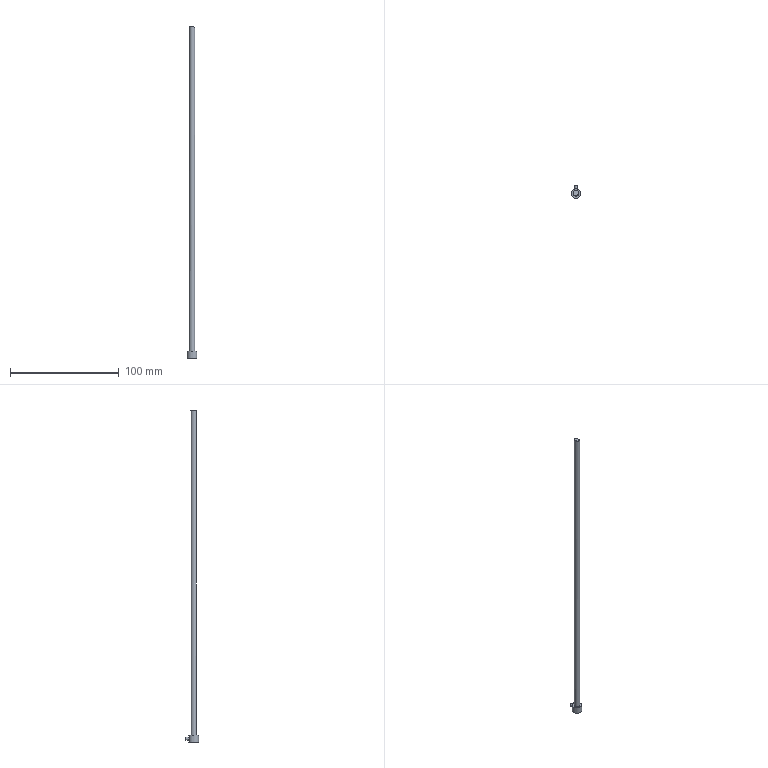Part | STEP file | E105-27-315 | 1 solid | 8 faces | box 9 x 12 x 304.744 mm | volume 6258 mm3 | cylinder 3 | plane 3 | spline 1 | cone 1 | commonest cylinder face diameters 3 x1 5 x1 9 x1
STEP:
#1=CARTESIAN_POINT('',(0.,0.,0.));
#2=DIRECTION('',(0.,0.,1.));
#3=DIRECTION('',(1.,0.,0.));
#4=AXIS2_PLACEMENT_3D('',#1,#2,#3);
#5=CARTESIAN_POINT('',(0.4483,-2.459,304.181));
#6=VERTEX_POINT('',#5);
#7=CARTESIAN_POINT('',(-2.5,0.,304.735));
#8=VERTEX_POINT('',#7);
#9=CARTESIAN_POINT('',(0.4483,-2.459,304.181));
#10=CARTESIAN_POINT('',(0.1679,-2.511,304.246));
#11=CARTESIAN_POINT('',(-0.1254,-2.513,304.312));
#12=CARTESIAN_POINT('',(-0.4075,-2.467,304.372));
#13=CARTESIAN_POINT('',(-0.6897,-2.42,304.433));
#14=CARTESIAN_POINT('',(-0.9686,-2.323,304.491));
#15=CARTESIAN_POINT('',(-1.22,-2.182,304.54));
#16=CARTESIAN_POINT('',(-1.468,-2.043,304.59));
#17=CARTESIAN_POINT('',(-1.697,-1.858,304.632));
#18=CARTESIAN_POINT('',(-1.885,-1.642,304.665));
#19=CARTESIAN_POINT('',(-2.069,-1.43,304.697));
#20=CARTESIAN_POINT('',(-2.22,-1.183,304.72));
#21=CARTESIAN_POINT('',(-2.324,-0.9216,304.732));
#22=CARTESIAN_POINT('',(-2.426,-0.6652,304.745));
#23=CARTESIAN_POINT('',(-2.485,-0.3875,304.747));
#24=CARTESIAN_POINT('',(-2.497,-0.1119,304.739));
#25=CARTESIAN_POINT('',(-2.51,0.1613,304.731));
#26=CARTESIAN_POINT('',(-2.476,0.4399,304.713));
#27=CARTESIAN_POINT('',(-2.4,0.7012,304.687));
#28=CARTESIAN_POINT('',(-2.323,0.9639,304.661));
#29=CARTESIAN_POINT('',(-2.201,1.216,304.625));
#30=CARTESIAN_POINT('',(-2.045,1.439,304.582));
#31=CARTESIAN_POINT('',(-1.886,1.665,304.539));
#32=CARTESIAN_POINT('',(-1.687,1.866,304.488));
#33=CARTESIAN_POINT('',(-1.464,2.026,304.434));
#34=CARTESIAN_POINT('',(-1.236,2.191,304.378));
#35=CARTESIAN_POINT('',(-0.9783,2.318,304.316));
#36=CARTESIAN_POINT('',(-0.7104,2.397,304.254));
#37=CARTESIAN_POINT('',(-0.4374,2.478,304.191));
#38=CARTESIAN_POINT('',(-0.1469,2.512,304.125));
#39=CARTESIAN_POINT('',(0.1375,2.496,304.062));
#40=CARTESIAN_POINT('',(0.424,2.48,303.999));
#41=CARTESIAN_POINT('',(0.7122,2.414,303.937));
#42=CARTESIAN_POINT('',(0.9777,2.301,303.881));
#43=CARTESIAN_POINT('',(1.241,2.189,303.826));
#44=CARTESIAN_POINT('',(1.489,2.029,303.776));
#45=CARTESIAN_POINT('',(1.701,1.832,303.735));
#46=CARTESIAN_POINT('',(1.907,1.64,303.695));
#47=CARTESIAN_POINT('',(2.085,1.409,303.663));
#48=CARTESIAN_POINT('',(2.216,1.157,303.643));
#49=CARTESIAN_POINT('',(2.344,0.9111,303.622));
#50=CARTESIAN_POINT('',(2.433,0.6393,303.612));
#51=CARTESIAN_POINT('',(2.473,0.3645,303.614));
#52=CARTESIAN_POINT('',(2.513,0.09415,303.615));
#53=CARTESIAN_POINT('',(2.508,-0.1866,303.627));
#54=CARTESIAN_POINT('',(2.458,-0.4544,303.648));
#55=CARTESIAN_POINT('',(2.409,-0.7223,303.67));
#56=CARTESIAN_POINT('',(2.314,-0.9846,303.702));
#57=CARTESIAN_POINT('',(2.182,-1.221,303.741));
#58=CARTESIAN_POINT('',(2.048,-1.46,303.781));
#59=CARTESIAN_POINT('',(1.872,-1.68,303.83));
#60=CARTESIAN_POINT('',(1.669,-1.862,303.883));
#61=CARTESIAN_POINT('',(1.46,-2.048,303.937));
#62=CARTESIAN_POINT('',(1.218,-2.201,303.998));
#63=CARTESIAN_POINT('',(0.9619,-2.308,304.06));
#64=CARTESIAN_POINT('',(0.797,-2.376,304.1));
#65=CARTESIAN_POINT('',(0.6239,-2.427,304.141));
#66=CARTESIAN_POINT('',(0.4483,-2.459,304.181));
#67=B_SPLINE_CURVE_WITH_KNOTS('',3,(#9,#10,#11,#12,#13,#14,#15,#16,#17,#18,#19,#20,#21,#22,#23,#24,#25,#26,#27,#28,#29,#30,#31,#32,#33,#34,#35,#36,#37,#38,#39,#40,#41,#42,#43,#44,#45,#46,#47,#48,#49,#50,#51,#52,#53,#54,#55,#56,#57,#58,#59,#60,#61,#62,#63,#64,#65,#66),.UNSPECIFIED.,.T.,.F.,(1,3,3,3,3,3,3,3,3,3,3,3,3,3,3,3,3,3,3,3,3,1),(-0.0344,0.,0.05541,0.1109,0.1656,0.2191,0.2714,0.3232,0.3753,0.4283,0.4826,0.5379,0.5936,0.6488,0.7029,0.7555,0.8073,0.8591,0.9117,0.9656,1.,1.055),.UNSPECIFIED.);
#68=CARTESIAN_POINT('',(0.,0.,106.));
#69=DIRECTION('',(0.,0.,-1.));
#70=DIRECTION('',(-1.,0.,0.));
#71=AXIS2_PLACEMENT_3D('',#68,#69,#70);
#72=CYLINDRICAL_SURFACE('',#71,2.5);
#73=CARTESIAN_POINT('',(4.532,-198.181));
#74=CARTESIAN_POINT('',(4.555,-198.195));
#75=CARTESIAN_POINT('',(4.602,-198.221));
#76=CARTESIAN_POINT('',(4.673,-198.261));
#77=CARTESIAN_POINT('',(4.744,-198.3));
#78=CARTESIAN_POINT('',(4.814,-198.339));
#79=CARTESIAN_POINT('',(4.885,-198.377));
#80=CARTESIAN_POINT('',(4.955,-198.414));
#81=CARTESIAN_POINT('',(5.026,-198.45));
#82=CARTESIAN_POINT('',(5.097,-198.484));
#83=CARTESIAN_POINT('',(5.169,-198.517));
#84=CARTESIAN_POINT('',(5.239,-198.548));
#85=CARTESIAN_POINT('',(5.311,-198.577));
#86=CARTESIAN_POINT('',(5.382,-198.605));
#87=CARTESIAN_POINT('',(5.454,-198.63));
#88=CARTESIAN_POINT('',(5.526,-198.653));
#89=CARTESIAN_POINT('',(5.597,-198.674));
#90=CARTESIAN_POINT('',(5.669,-198.692));
#91=CARTESIAN_POINT('',(5.741,-198.707));
#92=CARTESIAN_POINT('',(5.813,-198.72));
#93=CARTESIAN_POINT('',(5.886,-198.731));
#94=CARTESIAN_POINT('',(5.957,-198.738));
#95=CARTESIAN_POINT('',(6.03,-198.742));
#96=CARTESIAN_POINT('',(6.102,-198.744));
#97=CARTESIAN_POINT('',(6.175,-198.743));
#98=CARTESIAN_POINT('',(6.247,-198.739));
#99=CARTESIAN_POINT('',(6.319,-198.732));
#100=CARTESIAN_POINT('',(6.391,-198.722));
#101=CARTESIAN_POINT('',(6.464,-198.71));
#102=CARTESIAN_POINT('',(6.536,-198.695));
#103=CARTESIAN_POINT('',(6.607,-198.677));
#104=CARTESIAN_POINT('',(6.679,-198.657));
#105=CARTESIAN_POINT('',(6.751,-198.635));
#106=CARTESIAN_POINT('',(6.823,-198.61));
#107=CARTESIAN_POINT('',(6.894,-198.583));
#108=CARTESIAN_POINT('',(6.966,-198.555));
#109=CARTESIAN_POINT('',(7.037,-198.524));
#110=CARTESIAN_POINT('',(7.108,-198.492));
#111=CARTESIAN_POINT('',(7.179,-198.458));
#112=CARTESIAN_POINT('',(7.25,-198.423));
#113=CARTESIAN_POINT('',(7.321,-198.387));
#114=CARTESIAN_POINT('',(7.392,-198.35));
#115=CARTESIAN_POINT('',(7.463,-198.311));
#116=CARTESIAN_POINT('',(7.533,-198.273));
#117=CARTESIAN_POINT('',(7.603,-198.233));
#118=CARTESIAN_POINT('',(7.674,-198.194));
#119=CARTESIAN_POINT('',(7.745,-198.154));
#120=CARTESIAN_POINT('',(7.815,-198.114));
#121=CARTESIAN_POINT('',(7.886,-198.075));
#122=CARTESIAN_POINT('',(7.956,-198.036));
#123=CARTESIAN_POINT('',(8.027,-197.998));
#124=CARTESIAN_POINT('',(8.098,-197.961));
#125=CARTESIAN_POINT('',(8.168,-197.924));
#126=CARTESIAN_POINT('',(8.239,-197.889));
#127=CARTESIAN_POINT('',(8.31,-197.855));
#128=CARTESIAN_POINT('',(8.381,-197.823));
#129=CARTESIAN_POINT('',(8.452,-197.792));
#130=CARTESIAN_POINT('',(8.524,-197.763));
#131=CARTESIAN_POINT('',(8.595,-197.737));
#132=CARTESIAN_POINT('',(8.667,-197.713));
#133=CARTESIAN_POINT('',(8.738,-197.691));
#134=CARTESIAN_POINT('',(8.811,-197.671));
#135=CARTESIAN_POINT('',(8.883,-197.654));
#136=CARTESIAN_POINT('',(8.954,-197.64));
#137=CARTESIAN_POINT('',(9.026,-197.629));
#138=CARTESIAN_POINT('',(9.099,-197.621));
#139=CARTESIAN_POINT('',(9.171,-197.615));
#140=CARTESIAN_POINT('',(9.244,-197.613));
#141=CARTESIAN_POINT('',(9.315,-197.614));
#142=CARTESIAN_POINT('',(9.388,-197.618));
#143=CARTESIAN_POINT('',(9.46,-197.625));
#144=CARTESIAN_POINT('',(9.533,-197.634));
#145=CARTESIAN_POINT('',(9.605,-197.647));
#146=CARTESIAN_POINT('',(9.676,-197.663));
#147=CARTESIAN_POINT('',(9.749,-197.681));
#148=CARTESIAN_POINT('',(9.821,-197.702));
#149=CARTESIAN_POINT('',(9.892,-197.726));
#150=CARTESIAN_POINT('',(9.964,-197.751));
#151=CARTESIAN_POINT('',(10.035,-197.779));
#152=CARTESIAN_POINT('',(10.107,-197.809));
#153=CARTESIAN_POINT('',(10.178,-197.841));
#154=CARTESIAN_POINT('',(10.249,-197.875));
#155=CARTESIAN_POINT('',(10.32,-197.91));
#156=CARTESIAN_POINT('',(10.39,-197.946));
#157=CARTESIAN_POINT('',(10.461,-197.984));
#158=CARTESIAN_POINT('',(10.532,-198.022));
#159=CARTESIAN_POINT('',(10.602,-198.061));
#160=CARTESIAN_POINT('',(10.673,-198.101));
#161=CARTESIAN_POINT('',(10.744,-198.141));
#162=CARTESIAN_POINT('',(10.792,-198.168));
#163=CARTESIAN_POINT('',(10.815,-198.181));
#164=B_SPLINE_CURVE_WITH_KNOTS('',3,(#73,#74,#75,#76,#77,#78,#79,#80,#81,#82,#83,#84,#85,#86,#87,#88,#89,#90,#91,#92,#93,#94,#95,#96,#97,#98,#99,#100,#101,#102,#103,#104,#105,#106,#107,#108,#109,#110,#111,#112,#113,#114,#115,#116,#117,#118,#119,#120,#121,#122,#123,#124,#125,#126,#127,#128,#129,#130,#131,#132,#133,#134,#135,#136,#137,#138,#139,#140,#141,#142,#143,#144,#145,#146,#147,#148,#149,#150,#151,#152,#153,#154,#155,#156,#157,#158,#159,#160,#161,#162,#163),.UNSPECIFIED.,.F.,.F.,(4,1,1,1,1,1,1,1,1,1,1,1,1,1,1,1,1,1,1,1,1,1,1,1,1,1,1,1,1,1,1,1,1,1,1,1,1,1,1,1,1,1,1,1,1,1,1,1,1,1,1,1,1,1,1,1,1,1,1,1,1,1,1,1,1,1,1,1,1,1,1,1,1,1,1,1,1,1,1,1,1,1,1,1,1,1,1,1,4),(0.,0.01136,0.02273,0.03409,0.04545,0.05682,0.06818,0.07955,0.09091,0.1023,0.1136,0.125,0.1364,0.1477,0.1591,0.1705,0.1818,0.1932,0.2045,0.2159,0.2273,0.2386,0.25,0.2614,0.2727,0.2841,0.2955,0.3068,0.3182,0.3295,0.3409,0.3523,0.3636,0.375,0.3864,0.3977,0.4091,0.4205,0.4318,0.4432,0.4545,0.4659,0.4773,0.4886,0.5,0.5114,0.5227,0.5341,0.5455,0.5568,0.5682,0.5795,0.5909,0.6023,0.6136,0.625,0.6364,0.6477,0.6591,0.6705,0.6818,0.6932,0.7045,0.7159,0.7273,0.7386,0.75,0.7614,0.7727,0.7841,0.7955,0.8068,0.8182,0.8295,0.8409,0.8523,0.8636,0.875,0.8864,0.8977,0.9091,0.9205,0.9318,0.9432,0.9545,0.9659,0.9773,0.9886,1.),.QUASI_UNIFORM_KNOTS.);
#165=(GEOMETRIC_REPRESENTATION_CONTEXT(2)PARAMETRIC_REPRESENTATION_CONTEXT()REPRESENTATION_CONTEXT('',''));
#166=DEFINITIONAL_REPRESENTATION('',(#164),#165);
#167=PCURVE('',#72,#166);
#168=CARTESIAN_POINT('',(-8.095,-3.799,306.031));
#169=CARTESIAN_POINT('',(-2.709,-3.798,304.971));
#170=CARTESIAN_POINT('',(2.742,-3.796,303.756));
#171=CARTESIAN_POINT('',(8.261,-3.795,302.387));
#172=CARTESIAN_POINT('',(-8.134,-0.7578,305.924));
#173=CARTESIAN_POINT('',(-2.751,-0.7563,304.865));
#174=CARTESIAN_POINT('',(2.698,-0.7547,303.651));
#175=CARTESIAN_POINT('',(8.215,-0.7533,302.283));
#176=CARTESIAN_POINT('',(-8.175,2.283,305.817));
#177=CARTESIAN_POINT('',(-2.794,2.285,304.759));
#178=CARTESIAN_POINT('',(2.653,2.286,303.545));
#179=CARTESIAN_POINT('',(8.167,2.288,302.178));
#180=CARTESIAN_POINT('',(-8.216,5.325,305.709));
#181=CARTESIAN_POINT('',(-2.838,5.326,304.652));
#182=CARTESIAN_POINT('',(2.606,5.328,303.439));
#183=CARTESIAN_POINT('',(8.119,5.329,302.073));
#184=B_SPLINE_SURFACE_WITH_KNOTS('',3,3,((#168,#169,#170,#171),(#172,#173,#174,#175),(#176,#177,#178,#179),(#180,#181,#182,#183)),.UNSPECIFIED.,.F.,.F.,.F.,(4,4),(4,4),(0.,1.),(0.,1.),.PIECEWISE_BEZIER_KNOTS.);
#185=CARTESIAN_POINT('',(0.1466,0.5266));
#186=CARTESIAN_POINT('',(0.1459,0.5246));
#187=CARTESIAN_POINT('',(0.1448,0.5206));
#188=CARTESIAN_POINT('',(0.1435,0.5147));
#189=CARTESIAN_POINT('',(0.1426,0.5087));
#190=CARTESIAN_POINT('',(0.1422,0.5027));
#191=CARTESIAN_POINT('',(0.1421,0.4967));
#192=CARTESIAN_POINT('',(0.1425,0.4906));
#193=CARTESIAN_POINT('',(0.1433,0.4846));
#194=CARTESIAN_POINT('',(0.1445,0.4787));
#195=CARTESIAN_POINT('',(0.1462,0.4728));
#196=CARTESIAN_POINT('',(0.1483,0.4669));
#197=CARTESIAN_POINT('',(0.1508,0.461));
#198=CARTESIAN_POINT('',(0.1537,0.4552));
#199=CARTESIAN_POINT('',(0.157,0.4495));
#200=CARTESIAN_POINT('',(0.1607,0.4438));
#201=CARTESIAN_POINT('',(0.1649,0.4383));
#202=CARTESIAN_POINT('',(0.1694,0.4328));
#203=CARTESIAN_POINT('',(0.1743,0.4274));
#204=CARTESIAN_POINT('',(0.1795,0.4222));
#205=CARTESIAN_POINT('',(0.1852,0.417));
#206=CARTESIAN_POINT('',(0.1913,0.412));
#207=CARTESIAN_POINT('',(0.1977,0.4071));
#208=CARTESIAN_POINT('',(0.2045,0.4024));
#209=CARTESIAN_POINT('',(0.2116,0.3978));
#210=CARTESIAN_POINT('',(0.219,0.3934));
#211=CARTESIAN_POINT('',(0.2268,0.3891));
#212=CARTESIAN_POINT('',(0.2348,0.385));
#213=CARTESIAN_POINT('',(0.2431,0.3811));
#214=CARTESIAN_POINT('',(0.2518,0.3774));
#215=CARTESIAN_POINT('',(0.2607,0.3739));
#216=CARTESIAN_POINT('',(0.2699,0.3706));
#217=CARTESIAN_POINT('',(0.2794,0.3675));
#218=CARTESIAN_POINT('',(0.289,0.3646));
#219=CARTESIAN_POINT('',(0.2989,0.3619));
#220=CARTESIAN_POINT('',(0.3089,0.3594));
#221=CARTESIAN_POINT('',(0.3191,0.3572));
#222=CARTESIAN_POINT('',(0.3295,0.3553));
#223=CARTESIAN_POINT('',(0.34,0.3535));
#224=CARTESIAN_POINT('',(0.3507,0.352));
#225=CARTESIAN_POINT('',(0.3615,0.3507));
#226=CARTESIAN_POINT('',(0.3723,0.3497));
#227=CARTESIAN_POINT('',(0.3833,0.3489));
#228=CARTESIAN_POINT('',(0.3943,0.3484));
#229=CARTESIAN_POINT('',(0.4052,0.3481));
#230=CARTESIAN_POINT('',(0.4125,0.348));
#231=CARTESIAN_POINT('',(0.4162,0.3481));
#232=B_SPLINE_CURVE_WITH_KNOTS('',3,(#185,#186,#187,#188,#189,#190,#191,#192,#193,#194,#195,#196,#197,#198,#199,#200,#201,#202,#203,#204,#205,#206,#207,#208,#209,#210,#211,#212,#213,#214,#215,#216,#217,#218,#219,#220,#221,#222,#223,#224,#225,#226,#227,#228,#229,#230,#231),.UNSPECIFIED.,.F.,.F.,(4,1,1,1,1,1,1,1,1,1,1,1,1,1,1,1,1,1,1,1,1,1,1,1,1,1,1,1,1,1,1,1,1,1,1,1,1,1,1,1,1,1,1,1,4),(0.,0.006329,0.01266,0.01899,0.02531,0.03164,0.03797,0.0443,0.05063,0.05696,0.06329,0.06962,0.07594,0.08227,0.0886,0.09493,0.1013,0.1076,0.1139,0.1202,0.1266,0.1329,0.1392,0.1456,0.1519,0.1582,0.1645,0.1709,0.1772,0.1835,0.1899,0.1962,0.2025,0.2088,0.2152,0.2215,0.2278,0.2342,0.2405,0.2468,0.2531,0.2595,0.2658,0.2721,0.2785),.QUASI_UNIFORM_KNOTS.);
#233=(GEOMETRIC_REPRESENTATION_CONTEXT(2)PARAMETRIC_REPRESENTATION_CONTEXT()REPRESENTATION_CONTEXT('',''));
#234=DEFINITIONAL_REPRESENTATION('',(#232),#233);
#235=PCURVE('',#184,#234);
#236=SURFACE_CURVE('',#67,(#167,#235),.PCURVE_S1.);
#237=EDGE_CURVE('',#6,#8,#236,.T.);
#238=ORIENTED_EDGE('',*,*,#237,.T.);
#239=CARTESIAN_POINT('',(-2.5,0.,6.));
#240=VERTEX_POINT('',#239);
#241=CARTESIAN_POINT('',(-2.5,0.,304.735));
#242=CARTESIAN_POINT('',(-2.5,0.,6.));
#243=B_SPLINE_CURVE_WITH_KNOTS('',1,(#241,#242),.UNSPECIFIED.,.F.,.F.,(2,2),(-198.735,100.),.PIECEWISE_BEZIER_KNOTS.);
#244=CARTESIAN_POINT('',(6.283,0.));
#245=DIRECTION('',(0.,1.));
#246=VECTOR('',#245,1.);
#247=LINE('',#244,#246);
#248=(GEOMETRIC_REPRESENTATION_CONTEXT(2)PARAMETRIC_REPRESENTATION_CONTEXT()REPRESENTATION_CONTEXT('',''));
#249=DEFINITIONAL_REPRESENTATION('',(#247),#248);
#250=PCURVE('',#72,#249);
#251=CARTESIAN_POINT('',(0.,0.));
#252=DIRECTION('',(0.,1.));
#253=VECTOR('',#252,1.);
#254=LINE('',#251,#253);
#255=(GEOMETRIC_REPRESENTATION_CONTEXT(2)PARAMETRIC_REPRESENTATION_CONTEXT()REPRESENTATION_CONTEXT('',''));
#256=DEFINITIONAL_REPRESENTATION('',(#254),#255);
#257=PCURVE('',#72,#256);
#258=SEAM_CURVE('',#243,(#250,#257),.PCURVE_S1.);
#259=EDGE_CURVE('',#8,#240,#258,.T.);
#260=ORIENTED_EDGE('',*,*,#259,.T.);
#261=CARTESIAN_POINT('',(0.,0.,6.));
#262=DIRECTION('',(0.,0.,-1.));
#263=DIRECTION('',(-1.,0.,0.));
#264=AXIS2_PLACEMENT_3D('',#261,#262,#263);
#265=CIRCLE('',#264,2.5);
#266=CARTESIAN_POINT('',(0.,100.));
#267=DIRECTION('',(1.,0.));
#268=VECTOR('',#267,1.);
#269=LINE('',#266,#268);
#270=(GEOMETRIC_REPRESENTATION_CONTEXT(2)PARAMETRIC_REPRESENTATION_CONTEXT()REPRESENTATION_CONTEXT('',''));
#271=DEFINITIONAL_REPRESENTATION('',(#269),#270);
#272=PCURVE('',#72,#271);
#273=CARTESIAN_POINT('',(0.,0.,6.));
#274=DIRECTION('',(0.,0.,-1.));
#275=DIRECTION('',(1.,0.,0.));
#276=AXIS2_PLACEMENT_3D('',#273,#274,#275);
#277=PLANE('',#276);
#278=CARTESIAN_POINT('',(0.,0.));
#279=DIRECTION('',(-1.,0.));
#280=AXIS2_PLACEMENT_2D('',#278,#279);
#281=CIRCLE('',#280,2.5);
#282=(GEOMETRIC_REPRESENTATION_CONTEXT(2)PARAMETRIC_REPRESENTATION_CONTEXT()REPRESENTATION_CONTEXT('',''));
#283=DEFINITIONAL_REPRESENTATION('',(#281),#282);
#284=PCURVE('',#277,#283);
#285=SURFACE_CURVE('',#265,(#272,#284),.PCURVE_S1.);
#286=EDGE_CURVE('',#240,#240,#285,.T.);
#287=ORIENTED_EDGE('',*,*,#286,.F.);
#288=ORIENTED_EDGE('',*,*,#259,.F.);
#289=CARTESIAN_POINT('',(0.4483,-2.459,304.181));
#290=CARTESIAN_POINT('',(0.1679,-2.511,304.246));
#291=CARTESIAN_POINT('',(-0.1254,-2.513,304.312));
#292=CARTESIAN_POINT('',(-0.4075,-2.467,304.372));
#293=CARTESIAN_POINT('',(-0.6897,-2.42,304.433));
#294=CARTESIAN_POINT('',(-0.9686,-2.323,304.491));
#295=CARTESIAN_POINT('',(-1.22,-2.182,304.54));
#296=CARTESIAN_POINT('',(-1.468,-2.043,304.59));
#297=CARTESIAN_POINT('',(-1.697,-1.858,304.632));
#298=CARTESIAN_POINT('',(-1.885,-1.642,304.665));
#299=CARTESIAN_POINT('',(-2.069,-1.43,304.697));
#300=CARTESIAN_POINT('',(-2.22,-1.183,304.72));
#301=CARTESIAN_POINT('',(-2.324,-0.9216,304.732));
#302=CARTESIAN_POINT('',(-2.426,-0.6652,304.745));
#303=CARTESIAN_POINT('',(-2.485,-0.3875,304.747));
#304=CARTESIAN_POINT('',(-2.497,-0.1119,304.739));
#305=CARTESIAN_POINT('',(-2.51,0.1613,304.731));
#306=CARTESIAN_POINT('',(-2.476,0.4399,304.713));
#307=CARTESIAN_POINT('',(-2.4,0.7012,304.687));
#308=CARTESIAN_POINT('',(-2.323,0.9639,304.661));
#309=CARTESIAN_POINT('',(-2.201,1.216,304.625));
#310=CARTESIAN_POINT('',(-2.045,1.439,304.582));
#311=CARTESIAN_POINT('',(-1.886,1.665,304.539));
#312=CARTESIAN_POINT('',(-1.687,1.866,304.488));
#313=CARTESIAN_POINT('',(-1.464,2.026,304.434));
#314=CARTESIAN_POINT('',(-1.236,2.191,304.378));
#315=CARTESIAN_POINT('',(-0.9783,2.318,304.316));
#316=CARTESIAN_POINT('',(-0.7104,2.397,304.254));
#317=CARTESIAN_POINT('',(-0.4374,2.478,304.191));
#318=CARTESIAN_POINT('',(-0.1469,2.512,304.125));
#319=CARTESIAN_POINT('',(0.1375,2.496,304.062));
#320=CARTESIAN_POINT('',(0.424,2.48,303.999));
#321=CARTESIAN_POINT('',(0.7122,2.414,303.937));
#322=CARTESIAN_POINT('',(0.9777,2.301,303.881));
#323=CARTESIAN_POINT('',(1.241,2.189,303.826));
#324=CARTESIAN_POINT('',(1.489,2.029,303.776));
#325=CARTESIAN_POINT('',(1.701,1.832,303.735));
#326=CARTESIAN_POINT('',(1.907,1.64,303.695));
#327=CARTESIAN_POINT('',(2.085,1.409,303.663));
#328=CARTESIAN_POINT('',(2.216,1.157,303.643));
#329=CARTESIAN_POINT('',(2.344,0.9111,303.622));
#330=CARTESIAN_POINT('',(2.433,0.6393,303.612));
#331=CARTESIAN_POINT('',(2.473,0.3645,303.614));
#332=CARTESIAN_POINT('',(2.513,0.09415,303.615));
#333=CARTESIAN_POINT('',(2.508,-0.1866,303.627));
#334=CARTESIAN_POINT('',(2.458,-0.4544,303.648));
#335=CARTESIAN_POINT('',(2.409,-0.7223,303.67));
#336=CARTESIAN_POINT('',(2.314,-0.9846,303.702));
#337=CARTESIAN_POINT('',(2.182,-1.221,303.741));
#338=CARTESIAN_POINT('',(2.048,-1.46,303.781));
#339=CARTESIAN_POINT('',(1.872,-1.68,303.83));
#340=CARTESIAN_POINT('',(1.669,-1.862,303.883));
#341=CARTESIAN_POINT('',(1.46,-2.048,303.937));
#342=CARTESIAN_POINT('',(1.218,-2.201,303.998));
#343=CARTESIAN_POINT('',(0.9619,-2.308,304.06));
#344=CARTESIAN_POINT('',(0.797,-2.376,304.1));
#345=CARTESIAN_POINT('',(0.6239,-2.427,304.141));
#346=CARTESIAN_POINT('',(0.4483,-2.459,304.181));
#347=B_SPLINE_CURVE_WITH_KNOTS('',3,(#289,#290,#291,#292,#293,#294,#295,#296,#297,#298,#299,#300,#301,#302,#303,#304,#305,#306,#307,#308,#309,#310,#311,#312,#313,#314,#315,#316,#317,#318,#319,#320,#321,#322,#323,#324,#325,#326,#327,#328,#329,#330,#331,#332,#333,#334,#335,#336,#337,#338,#339,#340,#341,#342,#343,#344,#345,#346),.UNSPECIFIED.,.T.,.F.,(1,3,3,3,3,3,3,3,3,3,3,3,3,3,3,3,3,3,3,3,3,1),(-0.0344,0.,0.05541,0.1109,0.1656,0.2191,0.2714,0.3232,0.3753,0.4283,0.4826,0.5379,0.5936,0.6488,0.7029,0.7555,0.8073,0.8591,0.9117,0.9656,1.,1.055),.UNSPECIFIED.);
#348=CARTESIAN_POINT('',(-1.751,-198.181));
#349=CARTESIAN_POINT('',(-1.728,-198.195));
#350=CARTESIAN_POINT('',(-1.681,-198.221));
#351=CARTESIAN_POINT('',(-1.61,-198.261));
#352=CARTESIAN_POINT('',(-1.54,-198.3));
#353=CARTESIAN_POINT('',(-1.469,-198.339));
#354=CARTESIAN_POINT('',(-1.398,-198.377));
#355=CARTESIAN_POINT('',(-1.328,-198.414));
#356=CARTESIAN_POINT('',(-1.257,-198.45));
#357=CARTESIAN_POINT('',(-1.186,-198.484));
#358=CARTESIAN_POINT('',(-1.115,-198.517));
#359=CARTESIAN_POINT('',(-1.044,-198.548));
#360=CARTESIAN_POINT('',(-0.9726,-198.577));
#361=CARTESIAN_POINT('',(-0.901,-198.605));
#362=CARTESIAN_POINT('',(-0.8292,-198.63));
#363=CARTESIAN_POINT('',(-0.7575,-198.653));
#364=CARTESIAN_POINT('',(-0.6861,-198.674));
#365=CARTESIAN_POINT('',(-0.6142,-198.692));
#366=CARTESIAN_POINT('',(-0.542,-198.707));
#367=CARTESIAN_POINT('',(-0.4697,-198.72));
#368=CARTESIAN_POINT('',(-0.3976,-198.731));
#369=CARTESIAN_POINT('',(-0.3257,-198.738));
#370=CARTESIAN_POINT('',(-0.2533,-198.742));
#371=CARTESIAN_POINT('',(-0.1809,-198.744));
#372=CARTESIAN_POINT('',(-0.1084,-198.743));
#373=CARTESIAN_POINT('',(-0.03642,-198.739));
#374=CARTESIAN_POINT('',(0.03571,-198.732));
#375=CARTESIAN_POINT('',(0.1081,-198.722));
#376=CARTESIAN_POINT('',(0.1804,-198.71));
#377=CARTESIAN_POINT('',(0.2525,-198.695));
#378=CARTESIAN_POINT('',(0.3241,-198.677));
#379=CARTESIAN_POINT('',(0.3961,-198.657));
#380=CARTESIAN_POINT('',(0.468,-198.635));
#381=CARTESIAN_POINT('',(0.5398,-198.61));
#382=CARTESIAN_POINT('',(0.6112,-198.583));
#383=CARTESIAN_POINT('',(0.6823,-198.555));
#384=CARTESIAN_POINT('',(0.7537,-198.524));
#385=CARTESIAN_POINT('',(0.8251,-198.492));
#386=CARTESIAN_POINT('',(0.8962,-198.458));
#387=CARTESIAN_POINT('',(0.9668,-198.423));
#388=CARTESIAN_POINT('',(1.038,-198.387));
#389=CARTESIAN_POINT('',(1.108,-198.35));
#390=CARTESIAN_POINT('',(1.179,-198.311));
#391=CARTESIAN_POINT('',(1.25,-198.273));
#392=CARTESIAN_POINT('',(1.32,-198.233));
#393=CARTESIAN_POINT('',(1.391,-198.194));
#394=CARTESIAN_POINT('',(1.461,-198.154));
#395=CARTESIAN_POINT('',(1.532,-198.114));
#396=CARTESIAN_POINT('',(1.603,-198.075));
#397=CARTESIAN_POINT('',(1.673,-198.036));
#398=CARTESIAN_POINT('',(1.743,-197.998));
#399=CARTESIAN_POINT('',(1.814,-197.961));
#400=CARTESIAN_POINT('',(1.885,-197.924));
#401=CARTESIAN_POINT('',(1.956,-197.889));
#402=CARTESIAN_POINT('',(2.027,-197.855));
#403=CARTESIAN_POINT('',(2.098,-197.823));
#404=CARTESIAN_POINT('',(2.169,-197.792));
#405=CARTESIAN_POINT('',(2.241,-197.763));
#406=CARTESIAN_POINT('',(2.312,-197.737));
#407=CARTESIAN_POINT('',(2.383,-197.713));
#408=CARTESIAN_POINT('',(2.455,-197.691));
#409=CARTESIAN_POINT('',(2.527,-197.671));
#410=CARTESIAN_POINT('',(2.599,-197.654));
#411=CARTESIAN_POINT('',(2.671,-197.64));
#412=CARTESIAN_POINT('',(2.743,-197.629));
#413=CARTESIAN_POINT('',(2.816,-197.621));
#414=CARTESIAN_POINT('',(2.888,-197.615));
#415=CARTESIAN_POINT('',(2.96,-197.613));
#416=CARTESIAN_POINT('',(3.032,-197.614));
#417=CARTESIAN_POINT('',(3.105,-197.618));
#418=CARTESIAN_POINT('',(3.177,-197.625));
#419=CARTESIAN_POINT('',(3.249,-197.634));
#420=CARTESIAN_POINT('',(3.321,-197.647));
#421=CARTESIAN_POINT('',(3.393,-197.663));
#422=CARTESIAN_POINT('',(3.465,-197.681));
#423=CARTESIAN_POINT('',(3.537,-197.702));
#424=CARTESIAN_POINT('',(3.609,-197.726));
#425=CARTESIAN_POINT('',(3.68,-197.751));
#426=CARTESIAN_POINT('',(3.752,-197.779));
#427=CARTESIAN_POINT('',(3.823,-197.809));
#428=CARTESIAN_POINT('',(3.895,-197.841));
#429=CARTESIAN_POINT('',(3.966,-197.875));
#430=CARTESIAN_POINT('',(4.036,-197.91));
#431=CARTESIAN_POINT('',(4.107,-197.946));
#432=CARTESIAN_POINT('',(4.178,-197.984));
#433=CARTESIAN_POINT('',(4.249,-198.022));
#434=CARTESIAN_POINT('',(4.319,-198.061));
#435=CARTESIAN_POINT('',(4.39,-198.101));
#436=CARTESIAN_POINT('',(4.461,-198.141));
#437=CARTESIAN_POINT('',(4.508,-198.168));
#438=CARTESIAN_POINT('',(4.532,-198.181));
#439=B_SPLINE_CURVE_WITH_KNOTS('',3,(#348,#349,#350,#351,#352,#353,#354,#355,#356,#357,#358,#359,#360,#361,#362,#363,#364,#365,#366,#367,#368,#369,#370,#371,#372,#373,#374,#375,#376,#377,#378,#379,#380,#381,#382,#383,#384,#385,#386,#387,#388,#389,#390,#391,#392,#393,#394,#395,#396,#397,#398,#399,#400,#401,#402,#403,#404,#405,#406,#407,#408,#409,#410,#411,#412,#413,#414,#415,#416,#417,#418,#419,#420,#421,#422,#423,#424,#425,#426,#427,#428,#429,#430,#431,#432,#433,#434,#435,#436,#437,#438),.UNSPECIFIED.,.F.,.F.,(4,1,1,1,1,1,1,1,1,1,1,1,1,1,1,1,1,1,1,1,1,1,1,1,1,1,1,1,1,1,1,1,1,1,1,1,1,1,1,1,1,1,1,1,1,1,1,1,1,1,1,1,1,1,1,1,1,1,1,1,1,1,1,1,1,1,1,1,1,1,1,1,1,1,1,1,1,1,1,1,1,1,1,1,1,1,1,1,4),(0.,0.01136,0.02273,0.03409,0.04545,0.05682,0.06818,0.07955,0.09091,0.1023,0.1136,0.125,0.1364,0.1477,0.1591,0.1705,0.1818,0.1932,0.2045,0.2159,0.2273,0.2386,0.25,0.2614,0.2727,0.2841,0.2955,0.3068,0.3182,0.3295,0.3409,0.3523,0.3636,0.375,0.3864,0.3977,0.4091,0.4205,0.4318,0.4432,0.4545,0.4659,0.4773,0.4886,0.5,0.5114,0.5227,0.5341,0.5455,0.5568,0.5682,0.5795,0.5909,0.6023,0.6136,0.625,0.6364,0.6477,0.6591,0.6705,0.6818,0.6932,0.7045,0.7159,0.7273,0.7386,0.75,0.7614,0.7727,0.7841,0.7955,0.8068,0.8182,0.8295,0.8409,0.8523,0.8636,0.875,0.8864,0.8977,0.9091,0.9205,0.9318,0.9432,0.9545,0.9659,0.9773,0.9886,1.),.QUASI_UNIFORM_KNOTS.);
#440=(GEOMETRIC_REPRESENTATION_CONTEXT(2)PARAMETRIC_REPRESENTATION_CONTEXT()REPRESENTATION_CONTEXT('',''));
#441=DEFINITIONAL_REPRESENTATION('',(#439),#440);
#442=PCURVE('',#72,#441);
#443=CARTESIAN_POINT('',(0.4162,0.3481));
#444=CARTESIAN_POINT('',(0.4226,0.3481));
#445=CARTESIAN_POINT('',(0.4353,0.3485));
#446=CARTESIAN_POINT('',(0.4542,0.3498));
#447=CARTESIAN_POINT('',(0.473,0.3517));
#448=CARTESIAN_POINT('',(0.4914,0.3544));
#449=CARTESIAN_POINT('',(0.5094,0.3578));
#450=CARTESIAN_POINT('',(0.527,0.3619));
#451=CARTESIAN_POINT('',(0.5441,0.3667));
#452=CARTESIAN_POINT('',(0.5605,0.3721));
#453=CARTESIAN_POINT('',(0.5762,0.378));
#454=CARTESIAN_POINT('',(0.591,0.3846));
#455=CARTESIAN_POINT('',(0.6051,0.3917));
#456=CARTESIAN_POINT('',(0.6183,0.3993));
#457=CARTESIAN_POINT('',(0.6305,0.4074));
#458=CARTESIAN_POINT('',(0.6416,0.4158));
#459=CARTESIAN_POINT('',(0.6517,0.4247));
#460=CARTESIAN_POINT('',(0.6607,0.4339));
#461=CARTESIAN_POINT('',(0.6686,0.4435));
#462=CARTESIAN_POINT('',(0.6753,0.4533));
#463=CARTESIAN_POINT('',(0.6808,0.4632));
#464=CARTESIAN_POINT('',(0.685,0.4733));
#465=CARTESIAN_POINT('',(0.688,0.4836));
#466=CARTESIAN_POINT('',(0.6898,0.494));
#467=CARTESIAN_POINT('',(0.6904,0.5044));
#468=CARTESIAN_POINT('',(0.6896,0.5147));
#469=CARTESIAN_POINT('',(0.6876,0.525));
#470=CARTESIAN_POINT('',(0.6843,0.5353));
#471=CARTESIAN_POINT('',(0.6798,0.5454));
#472=CARTESIAN_POINT('',(0.6741,0.5552));
#473=CARTESIAN_POINT('',(0.6672,0.5648));
#474=CARTESIAN_POINT('',(0.6591,0.5742));
#475=CARTESIAN_POINT('',(0.6498,0.5832));
#476=CARTESIAN_POINT('',(0.6394,0.5919));
#477=CARTESIAN_POINT('',(0.6279,0.6001));
#478=CARTESIAN_POINT('',(0.6155,0.6078));
#479=CARTESIAN_POINT('',(0.6021,0.6151));
#480=CARTESIAN_POINT('',(0.5877,0.6219));
#481=CARTESIAN_POINT('',(0.5725,0.6281));
#482=CARTESIAN_POINT('',(0.5565,0.6337));
#483=CARTESIAN_POINT('',(0.5399,0.6386));
#484=CARTESIAN_POINT('',(0.5227,0.6429));
#485=CARTESIAN_POINT('',(0.5049,0.6466));
#486=CARTESIAN_POINT('',(0.4866,0.6495));
#487=CARTESIAN_POINT('',(0.468,0.6517));
#488=CARTESIAN_POINT('',(0.4492,0.6532));
#489=CARTESIAN_POINT('',(0.4302,0.654));
#490=CARTESIAN_POINT('',(0.4111,0.654));
#491=CARTESIAN_POINT('',(0.3921,0.6533));
#492=CARTESIAN_POINT('',(0.3732,0.6518));
#493=CARTESIAN_POINT('',(0.3546,0.6497));
#494=CARTESIAN_POINT('',(0.3362,0.6468));
#495=CARTESIAN_POINT('',(0.3183,0.6432));
#496=CARTESIAN_POINT('',(0.3008,0.639));
#497=CARTESIAN_POINT('',(0.2839,0.6341));
#498=CARTESIAN_POINT('',(0.2678,0.6286));
#499=CARTESIAN_POINT('',(0.2523,0.6225));
#500=CARTESIAN_POINT('',(0.2376,0.6159));
#501=CARTESIAN_POINT('',(0.2237,0.6087));
#502=CARTESIAN_POINT('',(0.2109,0.601));
#503=CARTESIAN_POINT('',(0.199,0.5929));
#504=CARTESIAN_POINT('',(0.1881,0.5844));
#505=CARTESIAN_POINT('',(0.1783,0.5755));
#506=CARTESIAN_POINT('',(0.1695,0.5662));
#507=CARTESIAN_POINT('',(0.162,0.5567));
#508=CARTESIAN_POINT('',(0.1555,0.5468));
#509=CARTESIAN_POINT('',(0.1503,0.5368));
#510=CARTESIAN_POINT('',(0.1477,0.53));
#511=CARTESIAN_POINT('',(0.1466,0.5266));
#512=B_SPLINE_CURVE_WITH_KNOTS('',3,(#443,#444,#445,#446,#447,#448,#449,#450,#451,#452,#453,#454,#455,#456,#457,#458,#459,#460,#461,#462,#463,#464,#465,#466,#467,#468,#469,#470,#471,#472,#473,#474,#475,#476,#477,#478,#479,#480,#481,#482,#483,#484,#485,#486,#487,#488,#489,#490,#491,#492,#493,#494,#495,#496,#497,#498,#499,#500,#501,#502,#503,#504,#505,#506,#507,#508,#509,#510,#511),.UNSPECIFIED.,.F.,.F.,(4,1,1,1,1,1,1,1,1,1,1,1,1,1,1,1,1,1,1,1,1,1,1,1,1,1,1,1,1,1,1,1,1,1,1,1,1,1,1,1,1,1,1,1,1,1,1,1,1,1,1,1,1,1,1,1,1,1,1,1,1,1,1,1,1,1,4),(0.2785,0.2894,0.3003,0.3113,0.3222,0.3331,0.3441,0.355,0.3659,0.3769,0.3878,0.3987,0.4097,0.4206,0.4315,0.4424,0.4534,0.4643,0.4752,0.4862,0.4971,0.508,0.519,0.5299,0.5408,0.5518,0.5627,0.5736,0.5846,0.5955,0.6064,0.6174,0.6283,0.6392,0.6502,0.6611,0.672,0.683,0.6939,0.7048,0.7158,0.7267,0.7376,0.7486,0.7595,0.7704,0.7814,0.7923,0.8032,0.8141,0.8251,0.836,0.8469,0.8579,0.8688,0.8797,0.8907,0.9016,0.9125,0.9235,0.9344,0.9453,0.9563,0.9672,0.9781,0.9891,1.),.QUASI_UNIFORM_KNOTS.);
#513=(GEOMETRIC_REPRESENTATION_CONTEXT(2)PARAMETRIC_REPRESENTATION_CONTEXT()REPRESENTATION_CONTEXT('',''));
#514=DEFINITIONAL_REPRESENTATION('',(#512),#513);
#515=PCURVE('',#184,#514);
#516=SURFACE_CURVE('',#347,(#442,#515),.PCURVE_S1.);
#517=EDGE_CURVE('',#8,#6,#516,.T.);
#518=ORIENTED_EDGE('',*,*,#517,.T.);
#519=EDGE_LOOP('',(#238,#260,#287,#288,#518));
#520=FACE_BOUND('',#519,.T.);
#521=ADVANCED_FACE('',(#520),#72,.T.);
#522=ORIENTED_EDGE('',*,*,#517,.T.);
#523=ORIENTED_EDGE('',*,*,#237,.T.);
#524=EDGE_LOOP('',(#522,#523));
#525=FACE_BOUND('',#524,.F.);
#526=ADVANCED_FACE('',(#525),#184,.F.);
#527=CARTESIAN_POINT('',(-4.5,0.,6.));
#528=VERTEX_POINT('',#527);
#529=CARTESIAN_POINT('',(0.,0.,6.));
#530=DIRECTION('',(0.,0.,-1.));
#531=DIRECTION('',(-1.,0.,0.));
#532=AXIS2_PLACEMENT_3D('',#529,#530,#531);
#533=CIRCLE('',#532,4.5);
#534=CARTESIAN_POINT('',(0.,0.));
#535=DIRECTION('',(-1.,0.));
#536=AXIS2_PLACEMENT_2D('',#534,#535);
#537=CIRCLE('',#536,4.5);
#538=(GEOMETRIC_REPRESENTATION_CONTEXT(2)PARAMETRIC_REPRESENTATION_CONTEXT()REPRESENTATION_CONTEXT('',''));
#539=DEFINITIONAL_REPRESENTATION('',(#537),#538);
#540=PCURVE('',#277,#539);
#541=CARTESIAN_POINT('',(0.,0.,-21.));
#542=DIRECTION('',(0.,0.,1.));
#543=DIRECTION('',(-1.,0.,0.));
#544=AXIS2_PLACEMENT_3D('',#541,#542,#543);
#545=CYLINDRICAL_SURFACE('',#544,4.5);
#546=CARTESIAN_POINT('',(6.283,27.));
#547=DIRECTION('',(-1.,0.));
#548=VECTOR('',#547,1.);
#549=LINE('',#546,#548);
#550=(GEOMETRIC_REPRESENTATION_CONTEXT(2)PARAMETRIC_REPRESENTATION_CONTEXT()REPRESENTATION_CONTEXT('',''));
#551=DEFINITIONAL_REPRESENTATION('',(#549),#550);
#552=PCURVE('',#545,#551);
#553=SURFACE_CURVE('',#533,(#540,#552),.PCURVE_S1.);
#554=EDGE_CURVE('',#528,#528,#553,.T.);
#555=ORIENTED_EDGE('',*,*,#554,.F.);
#556=EDGE_LOOP('',(#555));
#557=FACE_BOUND('',#556,.T.);
#558=ORIENTED_EDGE('',*,*,#286,.T.);
#559=EDGE_LOOP('',(#558));
#560=FACE_BOUND('',#559,.T.);
#561=ADVANCED_FACE('',(#557,#560),#277,.F.);
#562=CARTESIAN_POINT('',(4.5,0.,0.));
#563=VERTEX_POINT('',#562);
#564=CARTESIAN_POINT('',(-4.5,0.,0.));
#565=VERTEX_POINT('',#564);
#566=CARTESIAN_POINT('',(0.,0.,0.));
#567=DIRECTION('',(0.,0.,1.));
#568=DIRECTION('',(1.,0.,0.));
#569=AXIS2_PLACEMENT_3D('',#566,#567,#568);
#570=CIRCLE('',#569,4.5);
#571=CARTESIAN_POINT('',(3.142,21.));
#572=DIRECTION('',(1.,0.));
#573=VECTOR('',#572,1.);
#574=LINE('',#571,#573);
#575=(GEOMETRIC_REPRESENTATION_CONTEXT(2)PARAMETRIC_REPRESENTATION_CONTEXT()REPRESENTATION_CONTEXT('',''));
#576=DEFINITIONAL_REPRESENTATION('',(#574),#575);
#577=PCURVE('',#545,#576);
#578=CARTESIAN_POINT('',(320.,-1000.,0.));
#579=DIRECTION('',(0.,0.,1.));
#580=DIRECTION('',(-1.,0.,0.));
#581=AXIS2_PLACEMENT_3D('',#578,#579,#580);
#582=PLANE('',#581);
#583=CARTESIAN_POINT('',(320.,-1000.));
#584=DIRECTION('',(-1.,0.));
#585=AXIS2_PLACEMENT_2D('',#583,#584);
#586=CIRCLE('',#585,4.5);
#587=(GEOMETRIC_REPRESENTATION_CONTEXT(2)PARAMETRIC_REPRESENTATION_CONTEXT()REPRESENTATION_CONTEXT('',''));
#588=DEFINITIONAL_REPRESENTATION('',(#586),#587);
#589=PCURVE('',#582,#588);
#590=SURFACE_CURVE('',#570,(#577,#589),.PCURVE_S1.);
#591=EDGE_CURVE('',#563,#565,#590,.T.);
#592=ORIENTED_EDGE('',*,*,#591,.T.);
#593=CARTESIAN_POINT('',(-4.5,0.,0.));
#594=CARTESIAN_POINT('',(-4.5,0.,6.));
#595=B_SPLINE_CURVE_WITH_KNOTS('',1,(#593,#594),.UNSPECIFIED.,.F.,.F.,(2,2),(21.,27.),.PIECEWISE_BEZIER_KNOTS.);
#596=CARTESIAN_POINT('',(6.283,0.));
#597=DIRECTION('',(0.,1.));
#598=VECTOR('',#597,1.);
#599=LINE('',#596,#598);
#600=(GEOMETRIC_REPRESENTATION_CONTEXT(2)PARAMETRIC_REPRESENTATION_CONTEXT()REPRESENTATION_CONTEXT('',''));
#601=DEFINITIONAL_REPRESENTATION('',(#599),#600);
#602=PCURVE('',#545,#601);
#603=CARTESIAN_POINT('',(0.,0.));
#604=DIRECTION('',(0.,1.));
#605=VECTOR('',#604,1.);
#606=LINE('',#603,#605);
#607=(GEOMETRIC_REPRESENTATION_CONTEXT(2)PARAMETRIC_REPRESENTATION_CONTEXT()REPRESENTATION_CONTEXT('',''));
#608=DEFINITIONAL_REPRESENTATION('',(#606),#607);
#609=PCURVE('',#545,#608);
#610=SEAM_CURVE('',#595,(#602,#609),.PCURVE_S1.);
#611=EDGE_CURVE('',#565,#528,#610,.T.);
#612=ORIENTED_EDGE('',*,*,#611,.T.);
#613=ORIENTED_EDGE('',*,*,#554,.T.);
#614=ORIENTED_EDGE('',*,*,#611,.F.);
#615=CARTESIAN_POINT('',(0.,0.,0.));
#616=DIRECTION('',(0.,0.,1.));
#617=DIRECTION('',(1.,0.,0.));
#618=AXIS2_PLACEMENT_3D('',#615,#616,#617);
#619=CIRCLE('',#618,4.5);
#620=CARTESIAN_POINT('',(-3.142,21.));
#621=DIRECTION('',(1.,0.));
#622=VECTOR('',#621,1.);
#623=LINE('',#620,#622);
#624=(GEOMETRIC_REPRESENTATION_CONTEXT(2)PARAMETRIC_REPRESENTATION_CONTEXT()REPRESENTATION_CONTEXT('',''));
#625=DEFINITIONAL_REPRESENTATION('',(#623),#624);
#626=PCURVE('',#545,#625);
#627=CARTESIAN_POINT('',(320.,-1000.));
#628=DIRECTION('',(-1.,0.));
#629=AXIS2_PLACEMENT_2D('',#627,#628);
#630=CIRCLE('',#629,4.5);
#631=(GEOMETRIC_REPRESENTATION_CONTEXT(2)PARAMETRIC_REPRESENTATION_CONTEXT()REPRESENTATION_CONTEXT('',''));
#632=DEFINITIONAL_REPRESENTATION('',(#630),#631);
#633=PCURVE('',#582,#632);
#634=SURFACE_CURVE('',#619,(#626,#633),.PCURVE_S1.);
#635=EDGE_CURVE('',#565,#563,#634,.T.);
#636=ORIENTED_EDGE('',*,*,#635,.T.);
#637=EDGE_LOOP('',(#592,#612,#613,#614,#636));
#638=FACE_BOUND('',#637,.T.);
#639=CARTESIAN_POINT('',(0.,4.5,1.5));
#640=VERTEX_POINT('',#639);
#641=CARTESIAN_POINT('',(0.,4.5,1.5));
#642=CARTESIAN_POINT('',(-0.1629,4.5,1.5));
#643=CARTESIAN_POINT('',(-0.328,4.491,1.527));
#644=CARTESIAN_POINT('',(-0.4815,4.474,1.579));
#645=CARTESIAN_POINT('',(-0.6348,4.458,1.631));
#646=CARTESIAN_POINT('',(-0.7807,4.434,1.709));
#647=CARTESIAN_POINT('',(-0.9084,4.407,1.806));
#648=CARTESIAN_POINT('',(-1.04,4.38,1.907));
#649=CARTESIAN_POINT('',(-1.156,4.35,2.03));
#650=CARTESIAN_POINT('',(-1.248,4.323,2.168));
#651=CARTESIAN_POINT('',(-1.343,4.296,2.31));
#652=CARTESIAN_POINT('',(-1.414,4.272,2.471));
#653=CARTESIAN_POINT('',(-1.456,4.258,2.638));
#654=CARTESIAN_POINT('',(-1.496,4.244,2.799));
#655=CARTESIAN_POINT('',(-1.509,4.24,2.97));
#656=CARTESIAN_POINT('',(-1.494,4.245,3.136));
#657=CARTESIAN_POINT('',(-1.479,4.25,3.295));
#658=CARTESIAN_POINT('',(-1.439,4.264,3.452));
#659=CARTESIAN_POINT('',(-1.376,4.284,3.597));
#660=CARTESIAN_POINT('',(-1.312,4.305,3.744));
#661=CARTESIAN_POINT('',(-1.224,4.332,3.882));
#662=CARTESIAN_POINT('',(-1.117,4.359,4.001));
#663=CARTESIAN_POINT('',(-1.005,4.388,4.126));
#664=CARTESIAN_POINT('',(-0.8704,4.418,4.233));
#665=CARTESIAN_POINT('',(-0.7228,4.442,4.314));
#666=CARTESIAN_POINT('',(-0.5738,4.466,4.396));
#667=CARTESIAN_POINT('',(-0.4074,4.485,4.454));
#668=CARTESIAN_POINT('',(-0.238,4.494,4.481));
#669=CARTESIAN_POINT('',(-0.07599,4.502,4.507));
#670=CARTESIAN_POINT('',(0.09325,4.502,4.506));
#671=CARTESIAN_POINT('',(0.2549,4.493,4.478));
#672=CARTESIAN_POINT('',(0.4119,4.484,4.451));
#673=CARTESIAN_POINT('',(0.566,4.466,4.398));
#674=CARTESIAN_POINT('',(0.7055,4.444,4.324));
#675=CARTESIAN_POINT('',(0.8487,4.422,4.247));
#676=CARTESIAN_POINT('',(0.9804,4.393,4.147));
#677=CARTESIAN_POINT('',(1.091,4.366,4.029));
#678=CARTESIAN_POINT('',(1.207,4.337,3.906));
#679=CARTESIAN_POINT('',(1.303,4.308,3.762));
#680=CARTESIAN_POINT('',(1.372,4.286,3.606));
#681=CARTESIAN_POINT('',(1.44,4.264,3.451));
#682=CARTESIAN_POINT('',(1.483,4.249,3.281));
#683=CARTESIAN_POINT('',(1.496,4.244,3.111));
#684=CARTESIAN_POINT('',(1.508,4.24,2.949));
#685=CARTESIAN_POINT('',(1.493,4.245,2.783));
#686=CARTESIAN_POINT('',(1.453,4.259,2.627));
#687=CARTESIAN_POINT('',(1.413,4.272,2.473));
#688=CARTESIAN_POINT('',(1.349,4.294,2.325));
#689=CARTESIAN_POINT('',(1.264,4.319,2.193));
#690=CARTESIAN_POINT('',(1.176,4.345,2.054));
#691=CARTESIAN_POINT('',(1.064,4.374,1.93));
#692=CARTESIAN_POINT('',(0.9357,4.402,1.828));
#693=CARTESIAN_POINT('',(0.8027,4.43,1.721));
#694=CARTESIAN_POINT('',(0.6489,4.456,1.637));
#695=CARTESIAN_POINT('',(0.4866,4.474,1.581));
#696=CARTESIAN_POINT('',(0.3317,4.49,1.528));
#697=CARTESIAN_POINT('',(0.1647,4.5,1.5));
#698=CARTESIAN_POINT('',(0.,4.5,1.5));
#699=B_SPLINE_CURVE_WITH_KNOTS('',3,(#641,#642,#643,#644,#645,#646,#647,#648,#649,#650,#651,#652,#653,#654,#655,#656,#657,#658,#659,#660,#661,#662,#663,#664,#665,#666,#667,#668,#669,#670,#671,#672,#673,#674,#675,#676,#677,#678,#679,#680,#681,#682,#683,#684,#685,#686,#687,#688,#689,#690,#691,#692,#693,#694,#695,#696,#697,#698),.UNSPECIFIED.,.T.,.F.,(1,3,3,3,3,3,3,3,3,3,3,3,3,3,3,3,3,3,3,3,3,1),(-0.0523,0.,0.05173,0.1034,0.1566,0.2115,0.2645,0.3149,0.3662,0.4203,0.4749,0.5271,0.5777,0.6297,0.6841,0.7384,0.7898,0.8403,0.8929,0.9477,1.,1.052),.UNSPECIFIED.);
#700=CARTESIAN_POINT('',(4.712,22.5));
#701=CARTESIAN_POINT('',(4.72,22.5));
#702=CARTESIAN_POINT('',(4.736,22.503));
#703=CARTESIAN_POINT('',(4.76,22.514));
#704=CARTESIAN_POINT('',(4.784,22.534));
#705=CARTESIAN_POINT('',(4.807,22.56));
#706=CARTESIAN_POINT('',(4.83,22.594));
#707=CARTESIAN_POINT('',(4.852,22.636));
#708=CARTESIAN_POINT('',(4.873,22.684));
#709=CARTESIAN_POINT('',(4.894,22.738));
#710=CARTESIAN_POINT('',(4.914,22.799));
#711=CARTESIAN_POINT('',(4.933,22.866));
#712=CARTESIAN_POINT('',(4.951,22.939));
#713=CARTESIAN_POINT('',(4.967,23.017));
#714=CARTESIAN_POINT('',(4.983,23.1));
#715=CARTESIAN_POINT('',(4.997,23.187));
#716=CARTESIAN_POINT('',(5.009,23.278));
#717=CARTESIAN_POINT('',(5.02,23.374));
#718=CARTESIAN_POINT('',(5.03,23.473));
#719=CARTESIAN_POINT('',(5.038,23.575));
#720=CARTESIAN_POINT('',(5.044,23.678));
#721=CARTESIAN_POINT('',(5.049,23.784));
#722=CARTESIAN_POINT('',(5.052,23.892));
#723=CARTESIAN_POINT('',(5.052,24.));
#724=CARTESIAN_POINT('',(5.052,24.107));
#725=CARTESIAN_POINT('',(5.049,24.214));
#726=CARTESIAN_POINT('',(5.044,24.32));
#727=CARTESIAN_POINT('',(5.038,24.425));
#728=CARTESIAN_POINT('',(5.03,24.527));
#729=CARTESIAN_POINT('',(5.021,24.626));
#730=CARTESIAN_POINT('',(5.009,24.721));
#731=CARTESIAN_POINT('',(4.997,24.813));
#732=CARTESIAN_POINT('',(4.983,24.901));
#733=CARTESIAN_POINT('',(4.967,24.984));
#734=CARTESIAN_POINT('',(4.951,25.061));
#735=CARTESIAN_POINT('',(4.933,25.134));
#736=CARTESIAN_POINT('',(4.914,25.201));
#737=CARTESIAN_POINT('',(4.894,25.262));
#738=CARTESIAN_POINT('',(4.874,25.316));
#739=CARTESIAN_POINT('',(4.852,25.364));
#740=CARTESIAN_POINT('',(4.83,25.405));
#741=CARTESIAN_POINT('',(4.807,25.44));
#742=CARTESIAN_POINT('',(4.784,25.466));
#743=CARTESIAN_POINT('',(4.76,25.486));
#744=CARTESIAN_POINT('',(4.737,25.497));
#745=CARTESIAN_POINT('',(4.713,25.501));
#746=CARTESIAN_POINT('',(4.689,25.497));
#747=CARTESIAN_POINT('',(4.665,25.486));
#748=CARTESIAN_POINT('',(4.641,25.467));
#749=CARTESIAN_POINT('',(4.618,25.44));
#750=CARTESIAN_POINT('',(4.595,25.406));
#751=CARTESIAN_POINT('',(4.573,25.364));
#752=CARTESIAN_POINT('',(4.551,25.317));
#753=CARTESIAN_POINT('',(4.531,25.262));
#754=CARTESIAN_POINT('',(4.511,25.201));
#755=CARTESIAN_POINT('',(4.492,25.134));
#756=CARTESIAN_POINT('',(4.474,25.061));
#757=CARTESIAN_POINT('',(4.458,24.984));
#758=CARTESIAN_POINT('',(4.442,24.901));
#759=CARTESIAN_POINT('',(4.428,24.813));
#760=CARTESIAN_POINT('',(4.416,24.721));
#761=CARTESIAN_POINT('',(4.404,24.626));
#762=CARTESIAN_POINT('',(4.395,24.528));
#763=CARTESIAN_POINT('',(4.387,24.426));
#764=CARTESIAN_POINT('',(4.38,24.321));
#765=CARTESIAN_POINT('',(4.376,24.215));
#766=CARTESIAN_POINT('',(4.373,24.109));
#767=CARTESIAN_POINT('',(4.372,24.001));
#768=CARTESIAN_POINT('',(4.373,23.893));
#769=CARTESIAN_POINT('',(4.376,23.785));
#770=CARTESIAN_POINT('',(4.38,23.679));
#771=CARTESIAN_POINT('',(4.387,23.575));
#772=CARTESIAN_POINT('',(4.395,23.473));
#773=CARTESIAN_POINT('',(4.404,23.374));
#774=CARTESIAN_POINT('',(4.416,23.278));
#775=CARTESIAN_POINT('',(4.428,23.187));
#776=CARTESIAN_POINT('',(4.442,23.1));
#777=CARTESIAN_POINT('',(4.458,23.017));
#778=CARTESIAN_POINT('',(4.474,22.938));
#779=CARTESIAN_POINT('',(4.492,22.866));
#780=CARTESIAN_POINT('',(4.511,22.799));
#781=CARTESIAN_POINT('',(4.531,22.738));
#782=CARTESIAN_POINT('',(4.551,22.684));
#783=CARTESIAN_POINT('',(4.573,22.636));
#784=CARTESIAN_POINT('',(4.595,22.594));
#785=CARTESIAN_POINT('',(4.618,22.56));
#786=CARTESIAN_POINT('',(4.641,22.534));
#787=CARTESIAN_POINT('',(4.665,22.514));
#788=CARTESIAN_POINT('',(4.688,22.503));
#789=CARTESIAN_POINT('',(4.704,22.5));
#790=CARTESIAN_POINT('',(4.712,22.5));
#791=B_SPLINE_CURVE_WITH_KNOTS('',3,(#700,#701,#702,#703,#704,#705,#706,#707,#708,#709,#710,#711,#712,#713,#714,#715,#716,#717,#718,#719,#720,#721,#722,#723,#724,#725,#726,#727,#728,#729,#730,#731,#732,#733,#734,#735,#736,#737,#738,#739,#740,#741,#742,#743,#744,#745,#746,#747,#748,#749,#750,#751,#752,#753,#754,#755,#756,#757,#758,#759,#760,#761,#762,#763,#764,#765,#766,#767,#768,#769,#770,#771,#772,#773,#774,#775,#776,#777,#778,#779,#780,#781,#782,#783,#784,#785,#786,#787,#788,#789,#790),.UNSPECIFIED.,.T.,.F.,(4,1,1,1,1,1,1,1,1,1,1,1,1,1,1,1,1,1,1,1,1,1,1,1,1,1,1,1,1,1,1,1,1,1,1,1,1,1,1,1,1,1,1,1,1,1,1,1,1,1,1,1,1,1,1,1,1,1,1,1,1,1,1,1,1,1,1,1,1,1,1,1,1,1,1,1,1,1,1,1,1,1,1,1,1,1,1,1,4),(0.,0.01136,0.02273,0.03409,0.04545,0.05682,0.06818,0.07955,0.09091,0.1023,0.1136,0.125,0.1364,0.1477,0.1591,0.1705,0.1818,0.1932,0.2045,0.2159,0.2273,0.2386,0.25,0.2614,0.2727,0.2841,0.2955,0.3068,0.3182,0.3295,0.3409,0.3523,0.3636,0.375,0.3864,0.3977,0.4091,0.4205,0.4318,0.4432,0.4545,0.4659,0.4773,0.4886,0.5,0.5114,0.5227,0.5341,0.5455,0.5568,0.5682,0.5795,0.5909,0.6023,0.6136,0.625,0.6364,0.6477,0.6591,0.6705,0.6818,0.6932,0.7045,0.7159,0.7273,0.7386,0.75,0.7614,0.7727,0.7841,0.7955,0.8068,0.8182,0.8295,0.8409,0.8523,0.8636,0.875,0.8864,0.8977,0.9091,0.9205,0.9318,0.9432,0.9545,0.9659,0.9773,0.9886,1.),.QUASI_UNIFORM_KNOTS.);
#792=(GEOMETRIC_REPRESENTATION_CONTEXT(2)PARAMETRIC_REPRESENTATION_CONTEXT()REPRESENTATION_CONTEXT('',''));
#793=DEFINITIONAL_REPRESENTATION('',(#791),#792);
#794=PCURVE('',#545,#793);
#795=CARTESIAN_POINT('',(0.,-0.5,3.));
#796=DIRECTION('',(0.,1.,0.));
#797=DIRECTION('',(0.,0.,-1.));
#798=AXIS2_PLACEMENT_3D('',#795,#796,#797);
#799=CYLINDRICAL_SURFACE('',#798,1.5);
#800=CARTESIAN_POINT('',(0.,5.));
#801=CARTESIAN_POINT('',(0.02385,5.));
#802=CARTESIAN_POINT('',(0.07171,4.999));
#803=CARTESIAN_POINT('',(0.1437,4.995));
#804=CARTESIAN_POINT('',(0.2157,4.989));
#805=CARTESIAN_POINT('',(0.2875,4.98));
#806=CARTESIAN_POINT('',(0.3587,4.969));
#807=CARTESIAN_POINT('',(0.4301,4.957));
#808=CARTESIAN_POINT('',(0.5016,4.942));
#809=CARTESIAN_POINT('',(0.5729,4.926));
#810=CARTESIAN_POINT('',(0.6438,4.909));
#811=CARTESIAN_POINT('',(0.7145,4.891));
#812=CARTESIAN_POINT('',(0.7855,4.873));
#813=CARTESIAN_POINT('',(0.8566,4.855));
#814=CARTESIAN_POINT('',(0.9276,4.837));
#815=CARTESIAN_POINT('',(0.9983,4.82));
#816=CARTESIAN_POINT('',(1.069,4.803));
#817=CARTESIAN_POINT('',(1.141,4.788));
#818=CARTESIAN_POINT('',(1.212,4.775));
#819=CARTESIAN_POINT('',(1.284,4.764));
#820=CARTESIAN_POINT('',(1.355,4.754));
#821=CARTESIAN_POINT('',(1.427,4.748));
#822=CARTESIAN_POINT('',(1.499,4.744));
#823=CARTESIAN_POINT('',(1.571,4.742));
#824=CARTESIAN_POINT('',(1.642,4.744));
#825=CARTESIAN_POINT('',(1.714,4.748));
#826=CARTESIAN_POINT('',(1.786,4.754));
#827=CARTESIAN_POINT('',(1.858,4.764));
#828=CARTESIAN_POINT('',(1.929,4.775));
#829=CARTESIAN_POINT('',(2.001,4.788));
#830=CARTESIAN_POINT('',(2.072,4.803));
#831=CARTESIAN_POINT('',(2.143,4.82));
#832=CARTESIAN_POINT('',(2.214,4.837));
#833=CARTESIAN_POINT('',(2.285,4.855));
#834=CARTESIAN_POINT('',(2.356,4.873));
#835=CARTESIAN_POINT('',(2.427,4.891));
#836=CARTESIAN_POINT('',(2.498,4.909));
#837=CARTESIAN_POINT('',(2.569,4.926));
#838=CARTESIAN_POINT('',(2.64,4.942));
#839=CARTESIAN_POINT('',(2.711,4.956));
#840=CARTESIAN_POINT('',(2.782,4.969));
#841=CARTESIAN_POINT('',(2.854,4.98));
#842=CARTESIAN_POINT('',(2.926,4.989));
#843=CARTESIAN_POINT('',(2.997,4.995));
#844=CARTESIAN_POINT('',(3.069,4.999));
#845=CARTESIAN_POINT('',(3.141,5.));
#846=CARTESIAN_POINT('',(3.213,4.999));
#847=CARTESIAN_POINT('',(3.285,4.995));
#848=CARTESIAN_POINT('',(3.357,4.989));
#849=CARTESIAN_POINT('',(3.428,4.98));
#850=CARTESIAN_POINT('',(3.5,4.969));
#851=CARTESIAN_POINT('',(3.572,4.957));
#852=CARTESIAN_POINT('',(3.643,4.942));
#853=CARTESIAN_POINT('',(3.714,4.926));
#854=CARTESIAN_POINT('',(3.785,4.909));
#855=CARTESIAN_POINT('',(3.856,4.891));
#856=CARTESIAN_POINT('',(3.927,4.873));
#857=CARTESIAN_POINT('',(3.998,4.855));
#858=CARTESIAN_POINT('',(4.069,4.837));
#859=CARTESIAN_POINT('',(4.14,4.82));
#860=CARTESIAN_POINT('',(4.211,4.803));
#861=CARTESIAN_POINT('',(4.282,4.788));
#862=CARTESIAN_POINT('',(4.353,4.775));
#863=CARTESIAN_POINT('',(4.425,4.764));
#864=CARTESIAN_POINT('',(4.497,4.754));
#865=CARTESIAN_POINT('',(4.569,4.748));
#866=CARTESIAN_POINT('',(4.64,4.744));
#867=CARTESIAN_POINT('',(4.712,4.742));
#868=CARTESIAN_POINT('',(4.784,4.744));
#869=CARTESIAN_POINT('',(4.856,4.748));
#870=CARTESIAN_POINT('',(4.928,4.754));
#871=CARTESIAN_POINT('',(4.999,4.763));
#872=CARTESIAN_POINT('',(5.071,4.775));
#873=CARTESIAN_POINT('',(5.142,4.788));
#874=CARTESIAN_POINT('',(5.214,4.803));
#875=CARTESIAN_POINT('',(5.285,4.82));
#876=CARTESIAN_POINT('',(5.356,4.837));
#877=CARTESIAN_POINT('',(5.427,4.855));
#878=CARTESIAN_POINT('',(5.498,4.873));
#879=CARTESIAN_POINT('',(5.569,4.891));
#880=CARTESIAN_POINT('',(5.639,4.909));
#881=CARTESIAN_POINT('',(5.71,4.926));
#882=CARTESIAN_POINT('',(5.782,4.942));
#883=CARTESIAN_POINT('',(5.853,4.957));
#884=CARTESIAN_POINT('',(5.924,4.969));
#885=CARTESIAN_POINT('',(5.996,4.98));
#886=CARTESIAN_POINT('',(6.067,4.989));
#887=CARTESIAN_POINT('',(6.139,4.995));
#888=CARTESIAN_POINT('',(6.211,4.999));
#889=CARTESIAN_POINT('',(6.259,5.));
#890=CARTESIAN_POINT('',(6.283,5.));
#891=B_SPLINE_CURVE_WITH_KNOTS('',3,(#800,#801,#802,#803,#804,#805,#806,#807,#808,#809,#810,#811,#812,#813,#814,#815,#816,#817,#818,#819,#820,#821,#822,#823,#824,#825,#826,#827,#828,#829,#830,#831,#832,#833,#834,#835,#836,#837,#838,#839,#840,#841,#842,#843,#844,#845,#846,#847,#848,#849,#850,#851,#852,#853,#854,#855,#856,#857,#858,#859,#860,#861,#862,#863,#864,#865,#866,#867,#868,#869,#870,#871,#872,#873,#874,#875,#876,#877,#878,#879,#880,#881,#882,#883,#884,#885,#886,#887,#888,#889,#890),.UNSPECIFIED.,.F.,.F.,(4,1,1,1,1,1,1,1,1,1,1,1,1,1,1,1,1,1,1,1,1,1,1,1,1,1,1,1,1,1,1,1,1,1,1,1,1,1,1,1,1,1,1,1,1,1,1,1,1,1,1,1,1,1,1,1,1,1,1,1,1,1,1,1,1,1,1,1,1,1,1,1,1,1,1,1,1,1,1,1,1,1,1,1,1,1,1,1,4),(0.,0.01136,0.02273,0.03409,0.04545,0.05682,0.06818,0.07955,0.09091,0.1023,0.1136,0.125,0.1364,0.1477,0.1591,0.1705,0.1818,0.1932,0.2045,0.2159,0.2273,0.2386,0.25,0.2614,0.2727,0.2841,0.2955,0.3068,0.3182,0.3295,0.3409,0.3523,0.3636,0.375,0.3864,0.3977,0.4091,0.4205,0.4318,0.4432,0.4545,0.4659,0.4773,0.4886,0.5,0.5114,0.5227,0.5341,0.5455,0.5568,0.5682,0.5795,0.5909,0.6023,0.6136,0.625,0.6364,0.6477,0.6591,0.6705,0.6818,0.6932,0.7045,0.7159,0.7273,0.7386,0.75,0.7614,0.7727,0.7841,0.7955,0.8068,0.8182,0.8295,0.8409,0.8523,0.8636,0.875,0.8864,0.8977,0.9091,0.9205,0.9318,0.9432,0.9545,0.9659,0.9773,0.9886,1.),.QUASI_UNIFORM_KNOTS.);
#892=(GEOMETRIC_REPRESENTATION_CONTEXT(2)PARAMETRIC_REPRESENTATION_CONTEXT()REPRESENTATION_CONTEXT('',''));
#893=DEFINITIONAL_REPRESENTATION('',(#891),#892);
#894=PCURVE('',#799,#893);
#895=SURFACE_CURVE('',#699,(#794,#894),.PCURVE_S1.);
#896=EDGE_CURVE('',#640,#640,#895,.T.);
#897=ORIENTED_EDGE('',*,*,#896,.F.);
#898=EDGE_LOOP('',(#897));
#899=FACE_BOUND('',#898,.T.);
#900=ADVANCED_FACE('',(#638,#899),#545,.T.);
#901=ORIENTED_EDGE('',*,*,#591,.F.);
#902=ORIENTED_EDGE('',*,*,#635,.F.);
#903=EDGE_LOOP('',(#901,#902));
#904=FACE_BOUND('',#903,.T.);
#905=ADVANCED_FACE('',(#904),#582,.F.);
#906=CARTESIAN_POINT('',(0.,7.25,1.5));
#907=VERTEX_POINT('',#906);
#908=CARTESIAN_POINT('',(0.,7.25,3.));
#909=DIRECTION('',(0.,-1.,0.));
#910=DIRECTION('',(0.,0.,-1.));
#911=AXIS2_PLACEMENT_3D('',#908,#909,#910);
#912=CIRCLE('',#911,1.5);
#913=CARTESIAN_POINT('',(6.283,7.75));
#914=DIRECTION('',(-1.,0.));
#915=VECTOR('',#914,1.);
#916=LINE('',#913,#915);
#917=(GEOMETRIC_REPRESENTATION_CONTEXT(2)PARAMETRIC_REPRESENTATION_CONTEXT()REPRESENTATION_CONTEXT('',''));
#918=DEFINITIONAL_REPRESENTATION('',(#916),#917);
#919=PCURVE('',#799,#918);
#920=CARTESIAN_POINT('',(0.,7.25,3.));
#921=DIRECTION('',(0.,-1.,0.));
#922=DIRECTION('',(0.,0.,1.));
#923=AXIS2_PLACEMENT_3D('',#920,#921,#922);
#924=CONICAL_SURFACE('',#923,1.5,0.7854);
#925=CARTESIAN_POINT('',(3.142,0.));
#926=DIRECTION('',(1.,0.));
#927=VECTOR('',#926,1.);
#928=LINE('',#925,#927);
#929=(GEOMETRIC_REPRESENTATION_CONTEXT(2)PARAMETRIC_REPRESENTATION_CONTEXT()REPRESENTATION_CONTEXT('',''));
#930=DEFINITIONAL_REPRESENTATION('',(#928),#929);
#931=PCURVE('',#924,#930);
#932=SURFACE_CURVE('',#912,(#919,#931),.PCURVE_S1.);
#933=EDGE_CURVE('',#907,#907,#932,.T.);
#934=ORIENTED_EDGE('',*,*,#933,.T.);
#935=CARTESIAN_POINT('',(0.,4.5,1.5));
#936=CARTESIAN_POINT('',(0.,7.25,1.5));
#937=B_SPLINE_CURVE_WITH_KNOTS('',1,(#935,#936),.UNSPECIFIED.,.F.,.F.,(2,2),(5.,7.75),.PIECEWISE_BEZIER_KNOTS.);
#938=CARTESIAN_POINT('',(0.,0.));
#939=DIRECTION('',(0.,1.));
#940=VECTOR('',#939,1.);
#941=LINE('',#938,#940);
#942=(GEOMETRIC_REPRESENTATION_CONTEXT(2)PARAMETRIC_REPRESENTATION_CONTEXT()REPRESENTATION_CONTEXT('',''));
#943=DEFINITIONAL_REPRESENTATION('',(#941),#942);
#944=PCURVE('',#799,#943);
#945=CARTESIAN_POINT('',(6.283,0.));
#946=DIRECTION('',(0.,1.));
#947=VECTOR('',#946,1.);
#948=LINE('',#945,#947);
#949=(GEOMETRIC_REPRESENTATION_CONTEXT(2)PARAMETRIC_REPRESENTATION_CONTEXT()REPRESENTATION_CONTEXT('',''));
#950=DEFINITIONAL_REPRESENTATION('',(#948),#949);
#951=PCURVE('',#799,#950);
#952=SEAM_CURVE('',#937,(#944,#951),.PCURVE_S1.);
#953=EDGE_CURVE('',#640,#907,#952,.T.);
#954=ORIENTED_EDGE('',*,*,#953,.F.);
#955=ORIENTED_EDGE('',*,*,#896,.T.);
#956=ORIENTED_EDGE('',*,*,#953,.T.);
#957=EDGE_LOOP('',(#934,#954,#955,#956));
#958=FACE_BOUND('',#957,.T.);
#959=ADVANCED_FACE('',(#958),#799,.T.);
#960=CARTESIAN_POINT('',(0.,7.5,1.75));
#961=VERTEX_POINT('',#960);
#962=CARTESIAN_POINT('',(0.,7.5,3.));
#963=DIRECTION('',(0.,1.,0.));
#964=DIRECTION('',(0.,0.,-1.));
#965=AXIS2_PLACEMENT_3D('',#962,#963,#964);
#966=CIRCLE('',#965,1.25);
#967=CARTESIAN_POINT('',(0.,7.5,3.));
#968=DIRECTION('',(0.,1.,0.));
#969=DIRECTION('',(0.,0.,-1.));
#970=AXIS2_PLACEMENT_3D('',#967,#968,#969);
#971=PLANE('',#970);
#972=CARTESIAN_POINT('',(0.,0.));
#973=DIRECTION('',(1.,0.));
#974=AXIS2_PLACEMENT_2D('',#972,#973);
#975=CIRCLE('',#974,1.25);
#976=(GEOMETRIC_REPRESENTATION_CONTEXT(2)PARAMETRIC_REPRESENTATION_CONTEXT()REPRESENTATION_CONTEXT('',''));
#977=DEFINITIONAL_REPRESENTATION('',(#975),#976);
#978=PCURVE('',#971,#977);
#979=CARTESIAN_POINT('',(9.425,-0.25));
#980=DIRECTION('',(-1.,0.));
#981=VECTOR('',#980,1.);
#982=LINE('',#979,#981);
#983=(GEOMETRIC_REPRESENTATION_CONTEXT(2)PARAMETRIC_REPRESENTATION_CONTEXT()REPRESENTATION_CONTEXT('',''));
#984=DEFINITIONAL_REPRESENTATION('',(#982),#983);
#985=PCURVE('',#924,#984);
#986=SURFACE_CURVE('',#966,(#978,#985),.PCURVE_S1.);
#987=EDGE_CURVE('',#961,#961,#986,.T.);
#988=ORIENTED_EDGE('',*,*,#987,.T.);
#989=EDGE_LOOP('',(#988));
#990=FACE_BOUND('',#989,.T.);
#991=ADVANCED_FACE('',(#990),#971,.T.);
#992=ORIENTED_EDGE('',*,*,#987,.F.);
#993=CARTESIAN_POINT('',(0.,7.5,1.75));
#994=CARTESIAN_POINT('',(0.,7.25,1.5));
#995=B_SPLINE_CURVE_WITH_KNOTS('',1,(#993,#994),.UNSPECIFIED.,.F.,.F.,(2,2),(-0.3536,0.),.PIECEWISE_BEZIER_KNOTS.);
#996=CARTESIAN_POINT('',(9.425,0.));
#997=DIRECTION('',(0.,1.));
#998=VECTOR('',#997,1.);
#999=LINE('',#996,#998);
#1000=(GEOMETRIC_REPRESENTATION_CONTEXT(2)PARAMETRIC_REPRESENTATION_CONTEXT()REPRESENTATION_CONTEXT('',''));
#1001=DEFINITIONAL_REPRESENTATION('',(#999),#1000);
#1002=PCURVE('',#924,#1001);
#1003=CARTESIAN_POINT('',(3.142,0.));
#1004=DIRECTION('',(0.,1.));
#1005=VECTOR('',#1004,1.);
#1006=LINE('',#1003,#1005);
#1007=(GEOMETRIC_REPRESENTATION_CONTEXT(2)PARAMETRIC_REPRESENTATION_CONTEXT()REPRESENTATION_CONTEXT('',''));
#1008=DEFINITIONAL_REPRESENTATION('',(#1006),#1007);
#1009=PCURVE('',#924,#1008);
#1010=SEAM_CURVE('',#995,(#1002,#1009),.PCURVE_S1.);
#1011=EDGE_CURVE('',#961,#907,#1010,.T.);
#1012=ORIENTED_EDGE('',*,*,#1011,.T.);
#1013=ORIENTED_EDGE('',*,*,#933,.F.);
#1014=ORIENTED_EDGE('',*,*,#1011,.F.);
#1015=EDGE_LOOP('',(#992,#1012,#1013,#1014));
#1016=FACE_BOUND('',#1015,.T.);
#1017=ADVANCED_FACE('',(#1016),#924,.T.);
#1018=CLOSED_SHELL('',(#521,#526,#561,#900,#905,#959,#991,#1017));
#1019=MANIFOLD_SOLID_BREP('',#1018);
#1020=(LENGTH_UNIT()NAMED_UNIT(*)SI_UNIT(.MILLI.,.METRE.));
#1021=UNCERTAINTY_MEASURE_WITH_UNIT(LENGTH_MEASURE(0.00005),#1020,'','');
#1022=(NAMED_UNIT(*)PLANE_ANGLE_UNIT()SI_UNIT($,.RADIAN.));
#1023=(NAMED_UNIT(*)SI_UNIT($,.STERADIAN.)SOLID_ANGLE_UNIT());
#1024=(GEOMETRIC_REPRESENTATION_CONTEXT(3)GLOBAL_UNCERTAINTY_ASSIGNED_CONTEXT((#1021))GLOBAL_UNIT_ASSIGNED_CONTEXT((#1020,#1022,#1023))REPRESENTATION_CONTEXT('',''));
#1025=ADVANCED_BREP_SHAPE_REPRESENTATION('',(#4,#1019),#1024);